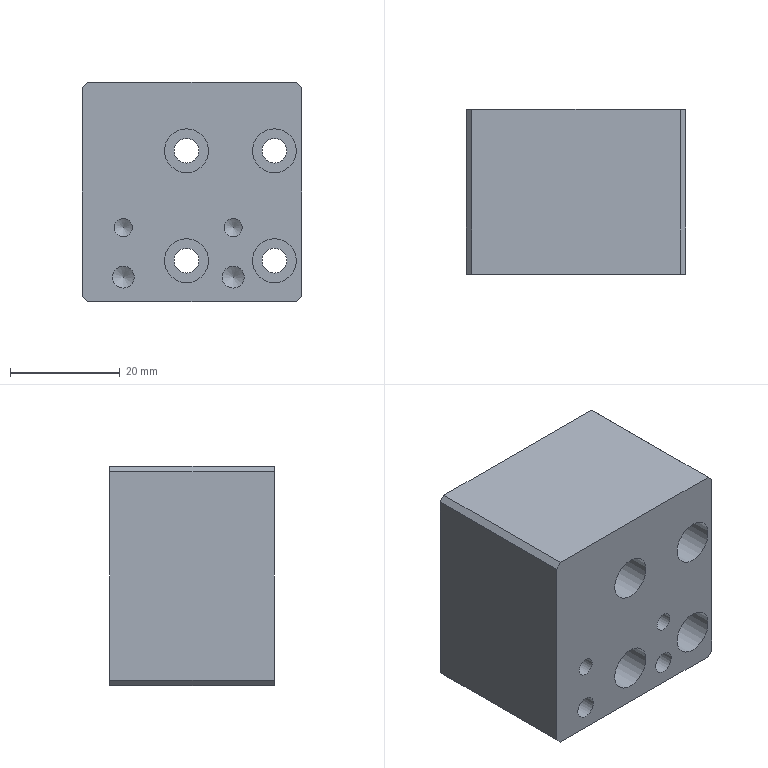CAM job | NX | 3+2 milling, drilling | part box 40 x 30 x 40 mm | stock box 45 x 35 x 45 mm
Tools:
number,name,description,diameter,corner_radius,flute_length,length,flutes
18,D2,平底铣刀-粗,2.0,0.0,50.0,75.0,2
4,D4,平底铣刀-粗,4.0,0.0,25.0,75.0,2
9,D10,平底铣刀-粗,10.0,0.0,35.0,75.0,2
19,D2-J,平底铣刀-精,2.0,0.0,50.0,75.0,2
17,D4-J,平底铣刀-精,4.0,0.0,50.0,75.0,2
10,D10-J,平底铣刀-精,10.0,0.0,35.0,75.0,2
1,D80R0.8飞刀,圆鼻刀-粗,80.0,0.8,50.0,75.0,2
2,D6倒角刀,倒角刀,6.0,0.0,3.0,25.0,2
21,M4X0.7,丝锥,3.3,0.0,35.0,50.0,2
13,ZT3.3,钻头,3.3,0.0,35.0,50.0,2
11,ZT4.5,钻头,4.5,0.0,35.0,50.0,2
13,钻头3.3,Twist Drill 3.3 mm,3.3,0.0,35.0,35.008,2
Operations:
program,operation,operation_type,tool,method,geometry_group,spindle_rpm,surface_speed,feed_per_tooth,feed_cut,feed_plunge,cut_length_mm,path_length_mm,cut_time_min,machine_time_min
A,顶面,FaceMilling,D80R0.8飞刀,侧刃精光-切深K-步距G,W-A,5000.0,1256.637,0.1,1000.0,100.0,134.0,170.0,0.134,0.1376
A,外形粗_2,VolumeBased25DMillingOperation,D10,METHOD,W-A,8000.0,251.327,0.3125,5000.0,80.0,7589.608,7658.408,1.518,1.525
A,打点-深0.8,Operation,D6倒角刀,NONE,W-A,8000.0,150.796,0.0312,500.0,90.0,14.4,155.593,0.0288,0.0429
A,盲锥孔-M4螺纹底孔,Operation,钻头3.3,NONE,W-A,3000.0,31.102,0.0417,250.0,90.0,24.183,109.391,0.0967,0.1053
A,盲锥孔-精孔4.0预钻,Operation,ZT3.3,NONE,W-A,3000.0,35.814,0.0417,250.0,90.0,24.403,109.832,0.0976,0.1062
A,沉头孔-钻孔0段,Operation,ZT4.5,NONE,W-A,2800.0,39.584,0.0357,200.0,90.0,137.408,369.903,0.687,0.7103
A,铣孔开粗D4_1,CylinderMilling,D4,NONE,W-A,8000.0,100.531,0.075,1200.0,100.0,4131.847,4441.847,3.443,3.474
A,铣孔精光D4_1,CylinderMilling,D4-J,精光步距切深关,W-A,8000.0,100.531,0.0312,500.0,100.0,351.069,661.069,0.7021,0.7331
A,铣孔开粗D2_1,CylinderMilling,D2,NONE,W-A,8000.0,50.266,0.0312,500.0,100.0,269.037,388.237,0.5381,0.55
A,仅选体,SurfaceContour,D6倒角刀,METHOD,W-A,8000.0,150.796,0.1875,3000.0,100.0,174.958,210.76,0.0583,0.0619
A,钻倒角_1,Operation,D6倒角刀,METHOD,W-A,8000.0,150.796,0.0312,500.0,0.0,10.4,84.024,0.0208,0.0282
A,钻倒角_2,Operation,D6倒角刀,METHOD,W-A,8000.0,150.796,0.0312,500.0,0.0,10.6,84.424,0.0212,0.0286
A,铣倒角_1,PlanarMilling,D6倒角刀,NONE,W-A,8000.0,150.796,0.0312,500.0,100.0,135.871,327.988,0.2717,0.291
A,盲锥孔-攻牙M4,Operation,M4X0.7,METHOD,W-A,800.0,8.294,0.0004,0.7,90.0,18.2,97.425,26.0,26.008
A,铣孔精光D2_1,CylinderMilling,D2-J,精光步距切深关,W-A,6000.0,37.699,0.0167,200.0,100.0,157.285,276.485,0.7864,0.7983
A,外形半精_2,VolumeBased25DMillingOperation,D10-J,METHOD,W-A,8000.0,251.327,0.0625,1000.0,100.0,388.062,559.476,0.3881,0.4052